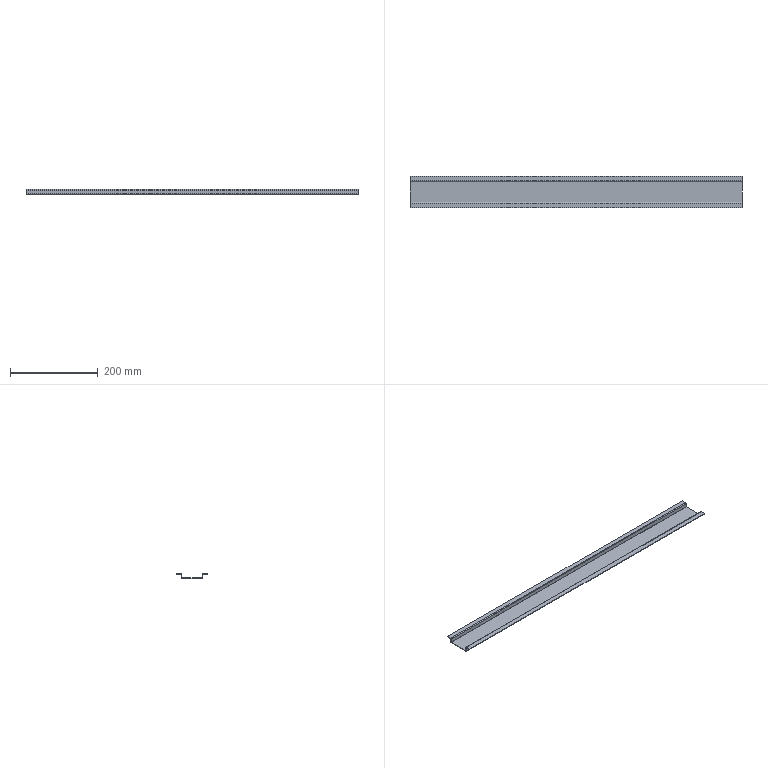Part | STEP file | FHD-0210-012-E side door A-F | 1 solid | 22 faces | box 757 x 71 x 12 mm | volume 102614 mm3 | plane 14 | cylinder 8 | commonest cylinder face diameters 0.4 x4 3.4 x4